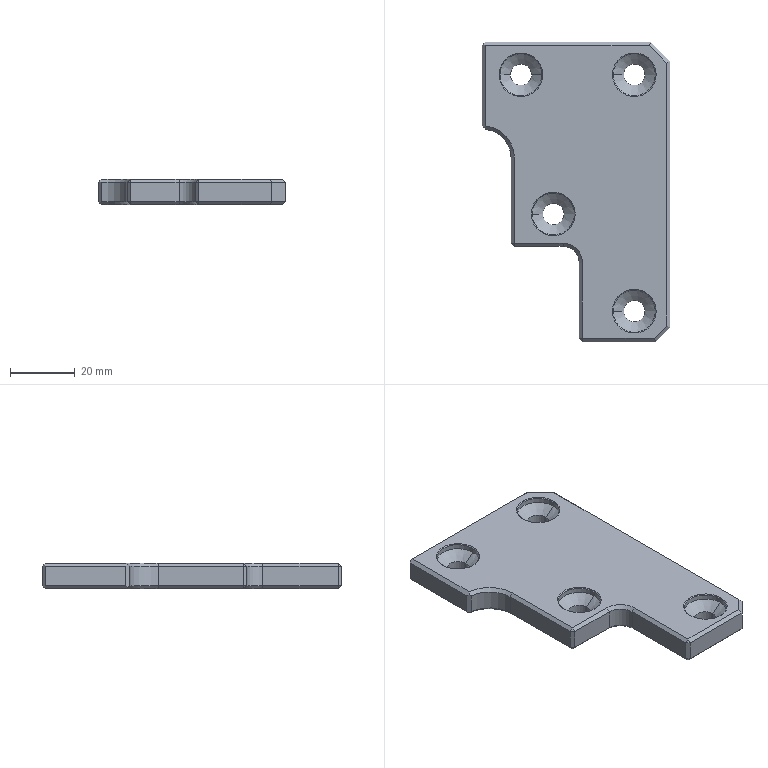Part | Creo | 1 solid | 77 faces | box 58 x 92.4 x 8 mm | volume 30632 mm3 | plane 39 | cone 20 | cylinder 18 | commonest cylinder face diameters 6.6 x8 13 x8 10 x1 18 x1